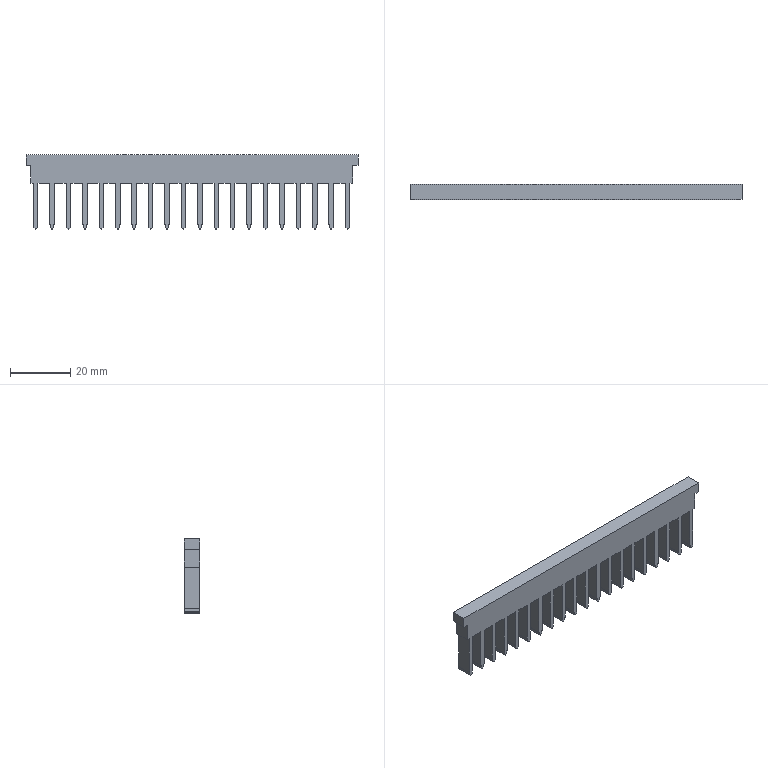Part | STEP file | 1 solid | 210 faces | box 110 x 5 x 24.6 mm | volume 7286 mm3 | plane 190 | cylinder 20 | commonest cylinder face diameters 0.48 x20